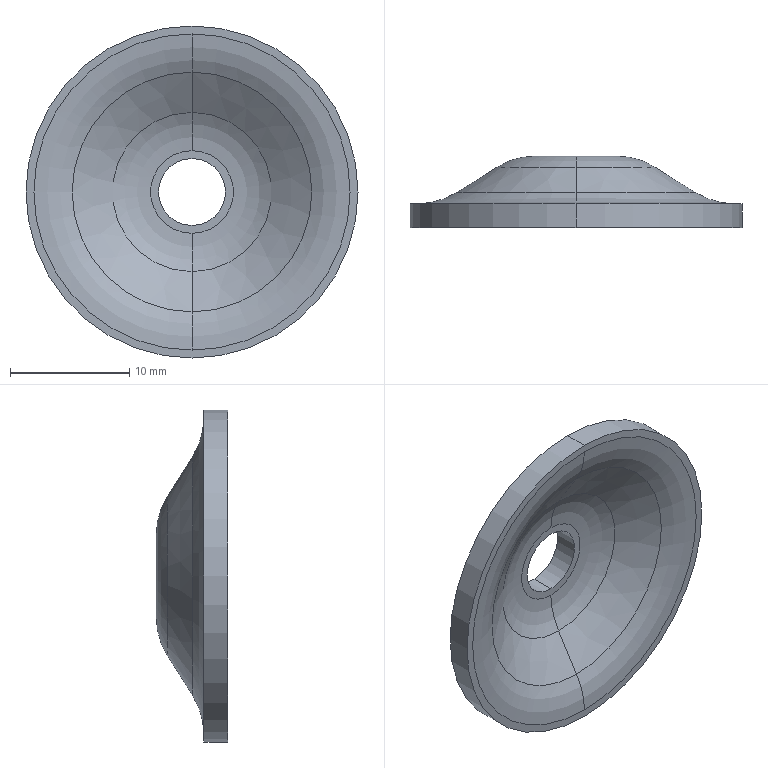Part | SolidWorks | features Revolution 1 | 1 solid | 20 faces | box 27.8 x 5.98 x 27.8 mm | volume 1165 mm3 | torus 8 | cone 4 | cylinder 4 | plane 4 | commonest cylinder face diameters 5.6 x2 27.8 x2
STEP:
#1=CARTESIAN_POINT('',(0.,-2.927,-6.668));
#2=VERTEX_POINT('',#1);
#3=CARTESIAN_POINT('',(0.,-2.927,6.668));
#4=VERTEX_POINT('',#3);
#5=CARTESIAN_POINT('',(0.,-2.927,0.));
#6=DIRECTION('',(0.,1.,0.));
#7=DIRECTION('',(0.,0.,1.));
#8=AXIS2_PLACEMENT_3D('',#5,#6,#7);
#9=CIRCLE('',#8,6.668);
#10=EDGE_CURVE('',#2,#4,#9,.T.);
#11=ORIENTED_EDGE('',*,*,#10,.F.);
#12=CARTESIAN_POINT('',(0.,-2.,-3.464));
#13=VERTEX_POINT('',#12);
#14=CARTESIAN_POINT('',(0.,-8.,-3.464));
#15=DIRECTION('',(1.,0.,0.));
#16=DIRECTION('',(0.,0.,-1.));
#17=AXIS2_PLACEMENT_3D('',#14,#15,#16);
#18=CIRCLE('',#17,6.);
#19=EDGE_CURVE('',#2,#13,#18,.T.);
#20=ORIENTED_EDGE('',*,*,#19,.T.);
#21=CARTESIAN_POINT('',(0.,-2.,3.464));
#22=VERTEX_POINT('',#21);
#23=CARTESIAN_POINT('',(0.,-2.,0.));
#24=DIRECTION('',(0.,1.,0.));
#25=DIRECTION('',(0.,0.,1.));
#26=AXIS2_PLACEMENT_3D('',#23,#24,#25);
#27=CIRCLE('',#26,3.464);
#28=EDGE_CURVE('',#13,#22,#27,.T.);
#29=ORIENTED_EDGE('',*,*,#28,.T.);
#30=CARTESIAN_POINT('',(0.,-8.,3.464));
#31=DIRECTION('',(-1.,0.,0.));
#32=DIRECTION('',(0.,0.,1.));
#33=AXIS2_PLACEMENT_3D('',#30,#31,#32);
#34=CIRCLE('',#33,6.);
#35=EDGE_CURVE('',#4,#22,#34,.T.);
#36=ORIENTED_EDGE('',*,*,#35,.F.);
#37=EDGE_LOOP('',(#11,#20,#29,#36));
#38=FACE_OUTER_BOUND('',#37,.T.);
#39=CARTESIAN_POINT('',(0.,-8.,0.));
#40=DIRECTION('',(0.,1.,0.));
#41=DIRECTION('',(0.,0.,1.));
#42=AXIS2_PLACEMENT_3D('',#39,#40,#41);
#43=TOROIDAL_SURFACE('',#42,3.464,6.);
#44=ADVANCED_FACE('',(#38),#43,.F.);
#45=ORIENTED_EDGE('',*,*,#10,.T.);
#46=CARTESIAN_POINT('',(0.,-5.053,10.032));
#47=VERTEX_POINT('',#46);
#48=CARTESIAN_POINT('',(0.,-5.053,10.032));
#49=DIRECTION('',(0.,-0.5341,0.8454));
#50=VECTOR('',#49,1000.);
#51=LINE('',#48,#50);
#52=EDGE_CURVE('',#4,#47,#51,.T.);
#53=ORIENTED_EDGE('',*,*,#52,.T.);
#54=CARTESIAN_POINT('',(0.,-5.053,-10.032));
#55=VERTEX_POINT('',#54);
#56=CARTESIAN_POINT('',(0.,-5.053,0.));
#57=DIRECTION('',(0.,1.,0.));
#58=DIRECTION('',(0.,0.,1.));
#59=AXIS2_PLACEMENT_3D('',#56,#57,#58);
#60=CIRCLE('',#59,10.032);
#61=EDGE_CURVE('',#55,#47,#60,.T.);
#62=ORIENTED_EDGE('',*,*,#61,.F.);
#63=CARTESIAN_POINT('',(0.,-5.053,-10.032));
#64=DIRECTION('',(0.,-0.5341,-0.8454));
#65=VECTOR('',#64,1000.);
#66=LINE('',#63,#65);
#67=EDGE_CURVE('',#2,#55,#66,.T.);
#68=ORIENTED_EDGE('',*,*,#67,.F.);
#69=EDGE_LOOP('',(#45,#53,#62,#68));
#70=FACE_OUTER_BOUND('',#69,.T.);
#71=CARTESIAN_POINT('',(0.,-5.053,0.));
#72=DIRECTION('',(0.,-1.,0.));
#73=DIRECTION('',(0.,0.,-1.));
#74=AXIS2_PLACEMENT_3D('',#71,#72,#73);
#75=CONICAL_SURFACE('',#74,10.032,1.007);
#76=ADVANCED_FACE('',(#70),#75,.F.);
#77=CARTESIAN_POINT('',(0.,-5.053,0.));
#78=DIRECTION('',(0.,1.,0.));
#79=DIRECTION('',(0.,0.,1.));
#80=AXIS2_PLACEMENT_3D('',#77,#78,#79);
#81=CIRCLE('',#80,10.032);
#82=EDGE_CURVE('',#47,#55,#81,.T.);
#83=ORIENTED_EDGE('',*,*,#82,.T.);
#84=CARTESIAN_POINT('',(0.,-5.98,-13.236));
#85=VERTEX_POINT('',#84);
#86=CARTESIAN_POINT('',(0.,0.02,-13.236));
#87=DIRECTION('',(1.,0.,0.));
#88=DIRECTION('',(0.,0.,-1.));
#89=AXIS2_PLACEMENT_3D('',#86,#87,#88);
#90=CIRCLE('',#89,6.);
#91=EDGE_CURVE('',#55,#85,#90,.T.);
#92=ORIENTED_EDGE('',*,*,#91,.T.);
#93=CARTESIAN_POINT('',(0.,-5.98,13.236));
#94=VERTEX_POINT('',#93);
#95=CARTESIAN_POINT('',(0.,-5.98,0.));
#96=DIRECTION('',(0.,1.,0.));
#97=DIRECTION('',(0.,0.,1.));
#98=AXIS2_PLACEMENT_3D('',#95,#96,#97);
#99=CIRCLE('',#98,13.236);
#100=EDGE_CURVE('',#94,#85,#99,.T.);
#101=ORIENTED_EDGE('',*,*,#100,.F.);
#102=CARTESIAN_POINT('',(0.,0.02,13.236));
#103=DIRECTION('',(-1.,0.,0.));
#104=DIRECTION('',(0.,0.,1.));
#105=AXIS2_PLACEMENT_3D('',#102,#103,#104);
#106=CIRCLE('',#105,6.);
#107=EDGE_CURVE('',#47,#94,#106,.T.);
#108=ORIENTED_EDGE('',*,*,#107,.F.);
#109=EDGE_LOOP('',(#83,#92,#101,#108));
#110=FACE_OUTER_BOUND('',#109,.T.);
#111=CARTESIAN_POINT('',(0.,0.02,0.));
#112=DIRECTION('',(0.,1.,0.));
#113=DIRECTION('',(0.,0.,1.));
#114=AXIS2_PLACEMENT_3D('',#111,#112,#113);
#115=TOROIDAL_SURFACE('',#114,13.236,6.);
#116=ADVANCED_FACE('',(#110),#115,.T.);
#117=CARTESIAN_POINT('',(0.,-5.98,13.9));
#118=VERTEX_POINT('',#117);
#119=CARTESIAN_POINT('',(0.,-5.98,-13.9));
#120=VERTEX_POINT('',#119);
#121=CARTESIAN_POINT('',(0.,-5.98,0.));
#122=DIRECTION('',(0.,1.,0.));
#123=DIRECTION('',(0.,0.,1.));
#124=AXIS2_PLACEMENT_3D('',#121,#122,#123);
#125=CIRCLE('',#124,13.9);
#126=EDGE_CURVE('',#118,#120,#125,.T.);
#127=ORIENTED_EDGE('',*,*,#126,.T.);
#128=CARTESIAN_POINT('',(0.,-3.98,-13.9));
#129=VERTEX_POINT('',#128);
#130=CARTESIAN_POINT('',(0.,0.,-13.9));
#131=DIRECTION('',(0.,1.,0.));
#132=VECTOR('',#131,1000.);
#133=LINE('',#130,#132);
#134=EDGE_CURVE('',#120,#129,#133,.T.);
#135=ORIENTED_EDGE('',*,*,#134,.T.);
#136=CARTESIAN_POINT('',(0.,-3.98,13.9));
#137=VERTEX_POINT('',#136);
#138=CARTESIAN_POINT('',(0.,-3.98,0.));
#139=DIRECTION('',(0.,1.,0.));
#140=DIRECTION('',(0.,0.,1.));
#141=AXIS2_PLACEMENT_3D('',#138,#139,#140);
#142=CIRCLE('',#141,13.9);
#143=EDGE_CURVE('',#137,#129,#142,.T.);
#144=ORIENTED_EDGE('',*,*,#143,.F.);
#145=CARTESIAN_POINT('',(0.,0.,13.9));
#146=DIRECTION('',(0.,1.,0.));
#147=VECTOR('',#146,1000.);
#148=LINE('',#145,#147);
#149=EDGE_CURVE('',#118,#137,#148,.T.);
#150=ORIENTED_EDGE('',*,*,#149,.F.);
#151=EDGE_LOOP('',(#127,#135,#144,#150));
#152=FACE_OUTER_BOUND('',#151,.T.);
#153=CARTESIAN_POINT('',(0.,0.,0.));
#154=DIRECTION('',(0.,1.,0.));
#155=DIRECTION('',(0.,0.,1.));
#156=AXIS2_PLACEMENT_3D('',#153,#154,#155);
#157=CYLINDRICAL_SURFACE('',#156,13.9);
#158=ADVANCED_FACE('',(#152),#157,.T.);
#159=CARTESIAN_POINT('',(0.,-3.053,-10.032));
#160=VERTEX_POINT('',#159);
#161=CARTESIAN_POINT('',(0.,-3.053,10.032));
#162=VERTEX_POINT('',#161);
#163=CARTESIAN_POINT('',(0.,-3.053,0.));
#164=DIRECTION('',(0.,1.,0.));
#165=DIRECTION('',(0.,0.,1.));
#166=AXIS2_PLACEMENT_3D('',#163,#164,#165);
#167=CIRCLE('',#166,10.032);
#168=EDGE_CURVE('',#160,#162,#167,.T.);
#169=ORIENTED_EDGE('',*,*,#168,.F.);
#170=CARTESIAN_POINT('',(0.,-3.98,-13.236));
#171=VERTEX_POINT('',#170);
#172=CARTESIAN_POINT('',(0.,2.02,-13.236));
#173=DIRECTION('',(1.,0.,0.));
#174=DIRECTION('',(0.,0.,-1.));
#175=AXIS2_PLACEMENT_3D('',#172,#173,#174);
#176=CIRCLE('',#175,6.);
#177=EDGE_CURVE('',#160,#171,#176,.T.);
#178=ORIENTED_EDGE('',*,*,#177,.T.);
#179=CARTESIAN_POINT('',(0.,-3.98,13.236));
#180=VERTEX_POINT('',#179);
#181=CARTESIAN_POINT('',(0.,-3.98,0.));
#182=DIRECTION('',(0.,1.,0.));
#183=DIRECTION('',(0.,0.,1.));
#184=AXIS2_PLACEMENT_3D('',#181,#182,#183);
#185=CIRCLE('',#184,13.236);
#186=EDGE_CURVE('',#171,#180,#185,.T.);
#187=ORIENTED_EDGE('',*,*,#186,.T.);
#188=CARTESIAN_POINT('',(0.,2.02,13.236));
#189=DIRECTION('',(-1.,0.,0.));
#190=DIRECTION('',(0.,0.,1.));
#191=AXIS2_PLACEMENT_3D('',#188,#189,#190);
#192=CIRCLE('',#191,6.);
#193=EDGE_CURVE('',#162,#180,#192,.T.);
#194=ORIENTED_EDGE('',*,*,#193,.F.);
#195=EDGE_LOOP('',(#169,#178,#187,#194));
#196=FACE_OUTER_BOUND('',#195,.T.);
#197=CARTESIAN_POINT('',(0.,2.02,0.));
#198=DIRECTION('',(0.,1.,0.));
#199=DIRECTION('',(0.,0.,1.));
#200=AXIS2_PLACEMENT_3D('',#197,#198,#199);
#201=TOROIDAL_SURFACE('',#200,13.236,6.);
#202=ADVANCED_FACE('',(#196),#201,.F.);
#203=CARTESIAN_POINT('',(0.,-0.9274,6.668));
#204=VERTEX_POINT('',#203);
#205=CARTESIAN_POINT('',(0.,-0.9274,-6.668));
#206=VERTEX_POINT('',#205);
#207=CARTESIAN_POINT('',(0.,-0.9274,0.));
#208=DIRECTION('',(0.,1.,0.));
#209=DIRECTION('',(0.,0.,1.));
#210=AXIS2_PLACEMENT_3D('',#207,#208,#209);
#211=CIRCLE('',#210,6.668);
#212=EDGE_CURVE('',#204,#206,#211,.T.);
#213=ORIENTED_EDGE('',*,*,#212,.F.);
#214=CARTESIAN_POINT('',(0.,-0.9274,6.668));
#215=DIRECTION('',(0.,-0.5341,0.8454));
#216=VECTOR('',#215,1000.);
#217=LINE('',#214,#216);
#218=EDGE_CURVE('',#204,#162,#217,.T.);
#219=ORIENTED_EDGE('',*,*,#218,.T.);
#220=CARTESIAN_POINT('',(0.,-3.053,0.));
#221=DIRECTION('',(0.,1.,0.));
#222=DIRECTION('',(0.,0.,1.));
#223=AXIS2_PLACEMENT_3D('',#220,#221,#222);
#224=CIRCLE('',#223,10.032);
#225=EDGE_CURVE('',#162,#160,#224,.T.);
#226=ORIENTED_EDGE('',*,*,#225,.T.);
#227=CARTESIAN_POINT('',(0.,-0.9274,-6.668));
#228=DIRECTION('',(0.,-0.5341,-0.8454));
#229=VECTOR('',#228,1000.);
#230=LINE('',#227,#229);
#231=EDGE_CURVE('',#206,#160,#230,.T.);
#232=ORIENTED_EDGE('',*,*,#231,.F.);
#233=EDGE_LOOP('',(#213,#219,#226,#232));
#234=FACE_OUTER_BOUND('',#233,.T.);
#235=CARTESIAN_POINT('',(0.,-0.9274,0.));
#236=DIRECTION('',(0.,-1.,0.));
#237=DIRECTION('',(0.,0.,-1.));
#238=AXIS2_PLACEMENT_3D('',#235,#236,#237);
#239=CONICAL_SURFACE('',#238,6.668,1.007);
#240=ADVANCED_FACE('',(#234),#239,.T.);
#241=ORIENTED_EDGE('',*,*,#212,.T.);
#242=CARTESIAN_POINT('',(0.,0.,-3.464));
#243=VERTEX_POINT('',#242);
#244=CARTESIAN_POINT('',(0.,-6.,-3.464));
#245=DIRECTION('',(1.,0.,0.));
#246=DIRECTION('',(0.,0.,-1.));
#247=AXIS2_PLACEMENT_3D('',#244,#245,#246);
#248=CIRCLE('',#247,6.);
#249=EDGE_CURVE('',#206,#243,#248,.T.);
#250=ORIENTED_EDGE('',*,*,#249,.T.);
#251=CARTESIAN_POINT('',(0.,0.,3.464));
#252=VERTEX_POINT('',#251);
#253=CARTESIAN_POINT('',(0.,0.,0.));
#254=DIRECTION('',(0.,1.,0.));
#255=DIRECTION('',(0.,0.,1.));
#256=AXIS2_PLACEMENT_3D('',#253,#254,#255);
#257=CIRCLE('',#256,3.464);
#258=EDGE_CURVE('',#252,#243,#257,.T.);
#259=ORIENTED_EDGE('',*,*,#258,.F.);
#260=CARTESIAN_POINT('',(0.,-6.,3.464));
#261=DIRECTION('',(-1.,0.,0.));
#262=DIRECTION('',(0.,0.,1.));
#263=AXIS2_PLACEMENT_3D('',#260,#261,#262);
#264=CIRCLE('',#263,6.);
#265=EDGE_CURVE('',#204,#252,#264,.T.);
#266=ORIENTED_EDGE('',*,*,#265,.F.);
#267=EDGE_LOOP('',(#241,#250,#259,#266));
#268=FACE_OUTER_BOUND('',#267,.T.);
#269=CARTESIAN_POINT('',(0.,-6.,0.));
#270=DIRECTION('',(0.,1.,0.));
#271=DIRECTION('',(0.,0.,1.));
#272=AXIS2_PLACEMENT_3D('',#269,#270,#271);
#273=TOROIDAL_SURFACE('',#272,3.464,6.);
#274=ADVANCED_FACE('',(#268),#273,.T.);
#275=CARTESIAN_POINT('',(0.,-2.,-2.8));
#276=VERTEX_POINT('',#275);
#277=CARTESIAN_POINT('',(0.,-2.,2.8));
#278=VERTEX_POINT('',#277);
#279=CARTESIAN_POINT('',(0.,-2.,0.));
#280=DIRECTION('',(0.,1.,0.));
#281=DIRECTION('',(0.,0.,1.));
#282=AXIS2_PLACEMENT_3D('',#279,#280,#281);
#283=CIRCLE('',#282,2.8);
#284=EDGE_CURVE('',#276,#278,#283,.T.);
#285=ORIENTED_EDGE('',*,*,#284,.F.);
#286=CARTESIAN_POINT('',(0.,0.,-2.8));
#287=VERTEX_POINT('',#286);
#288=CARTESIAN_POINT('',(0.,0.,-2.8));
#289=DIRECTION('',(0.,1.,0.));
#290=VECTOR('',#289,1000.);
#291=LINE('',#288,#290);
#292=EDGE_CURVE('',#276,#287,#291,.T.);
#293=ORIENTED_EDGE('',*,*,#292,.T.);
#294=CARTESIAN_POINT('',(0.,0.,2.8));
#295=VERTEX_POINT('',#294);
#296=CARTESIAN_POINT('',(0.,0.,0.));
#297=DIRECTION('',(0.,1.,0.));
#298=DIRECTION('',(0.,0.,1.));
#299=AXIS2_PLACEMENT_3D('',#296,#297,#298);
#300=CIRCLE('',#299,2.8);
#301=EDGE_CURVE('',#287,#295,#300,.T.);
#302=ORIENTED_EDGE('',*,*,#301,.T.);
#303=CARTESIAN_POINT('',(0.,0.,2.8));
#304=DIRECTION('',(0.,1.,0.));
#305=VECTOR('',#304,1000.);
#306=LINE('',#303,#305);
#307=EDGE_CURVE('',#278,#295,#306,.T.);
#308=ORIENTED_EDGE('',*,*,#307,.F.);
#309=EDGE_LOOP('',(#285,#293,#302,#308));
#310=FACE_OUTER_BOUND('',#309,.T.);
#311=CARTESIAN_POINT('',(0.,0.,0.));
#312=DIRECTION('',(0.,1.,0.));
#313=DIRECTION('',(0.,0.,1.));
#314=AXIS2_PLACEMENT_3D('',#311,#312,#313);
#315=CYLINDRICAL_SURFACE('',#314,2.8);
#316=ADVANCED_FACE('',(#310),#315,.F.);
#317=ORIENTED_EDGE('',*,*,#292,.F.);
#318=CARTESIAN_POINT('',(0.,-2.,0.));
#319=DIRECTION('',(0.,1.,0.));
#320=DIRECTION('',(0.,0.,1.));
#321=AXIS2_PLACEMENT_3D('',#318,#319,#320);
#322=CIRCLE('',#321,2.8);
#323=EDGE_CURVE('',#278,#276,#322,.T.);
#324=ORIENTED_EDGE('',*,*,#323,.F.);
#325=ORIENTED_EDGE('',*,*,#307,.T.);
#326=CARTESIAN_POINT('',(0.,0.,0.));
#327=DIRECTION('',(0.,1.,0.));
#328=DIRECTION('',(0.,0.,1.));
#329=AXIS2_PLACEMENT_3D('',#326,#327,#328);
#330=CIRCLE('',#329,2.8);
#331=EDGE_CURVE('',#295,#287,#330,.T.);
#332=ORIENTED_EDGE('',*,*,#331,.T.);
#333=EDGE_LOOP('',(#317,#324,#325,#332));
#334=FACE_OUTER_BOUND('',#333,.T.);
#335=CARTESIAN_POINT('',(0.,0.,0.));
#336=DIRECTION('',(0.,1.,0.));
#337=DIRECTION('',(0.,0.,1.));
#338=AXIS2_PLACEMENT_3D('',#335,#336,#337);
#339=CYLINDRICAL_SURFACE('',#338,2.8);
#340=ADVANCED_FACE('',(#334),#339,.F.);
#341=ORIENTED_EDGE('',*,*,#258,.T.);
#342=CARTESIAN_POINT('',(0.,0.,0.));
#343=DIRECTION('',(0.,1.,0.));
#344=DIRECTION('',(0.,0.,1.));
#345=AXIS2_PLACEMENT_3D('',#342,#343,#344);
#346=CIRCLE('',#345,3.464);
#347=EDGE_CURVE('',#243,#252,#346,.T.);
#348=ORIENTED_EDGE('',*,*,#347,.T.);
#349=EDGE_LOOP('',(#341,#348));
#350=FACE_OUTER_BOUND('',#349,.T.);
#351=ORIENTED_EDGE('',*,*,#331,.F.);
#352=ORIENTED_EDGE('',*,*,#301,.F.);
#353=EDGE_LOOP('',(#351,#352));
#354=FACE_BOUND('',#353,.T.);
#355=CARTESIAN_POINT('',(-2.8,0.,0.));
#356=DIRECTION('',(0.,1.,0.));
#357=DIRECTION('',(0.,0.,1.));
#358=AXIS2_PLACEMENT_3D('',#355,#356,#357);
#359=PLANE('',#358);
#360=ADVANCED_FACE('',(#350,#354),#359,.T.);
#361=ORIENTED_EDGE('',*,*,#249,.F.);
#362=CARTESIAN_POINT('',(0.,-0.9274,0.));
#363=DIRECTION('',(0.,1.,0.));
#364=DIRECTION('',(0.,0.,1.));
#365=AXIS2_PLACEMENT_3D('',#362,#363,#364);
#366=CIRCLE('',#365,6.668);
#367=EDGE_CURVE('',#206,#204,#366,.T.);
#368=ORIENTED_EDGE('',*,*,#367,.T.);
#369=ORIENTED_EDGE('',*,*,#265,.T.);
#370=ORIENTED_EDGE('',*,*,#347,.F.);
#371=EDGE_LOOP('',(#361,#368,#369,#370));
#372=FACE_OUTER_BOUND('',#371,.T.);
#373=CARTESIAN_POINT('',(0.,-6.,0.));
#374=DIRECTION('',(0.,1.,0.));
#375=DIRECTION('',(0.,0.,1.));
#376=AXIS2_PLACEMENT_3D('',#373,#374,#375);
#377=TOROIDAL_SURFACE('',#376,3.464,6.);
#378=ADVANCED_FACE('',(#372),#377,.T.);
#379=ORIENTED_EDGE('',*,*,#218,.F.);
#380=ORIENTED_EDGE('',*,*,#367,.F.);
#381=ORIENTED_EDGE('',*,*,#231,.T.);
#382=ORIENTED_EDGE('',*,*,#168,.T.);
#383=EDGE_LOOP('',(#379,#380,#381,#382));
#384=FACE_OUTER_BOUND('',#383,.T.);
#385=CARTESIAN_POINT('',(0.,-0.9274,0.));
#386=DIRECTION('',(0.,-1.,0.));
#387=DIRECTION('',(0.,0.,-1.));
#388=AXIS2_PLACEMENT_3D('',#385,#386,#387);
#389=CONICAL_SURFACE('',#388,6.668,1.007);
#390=ADVANCED_FACE('',(#384),#389,.T.);
#391=ORIENTED_EDGE('',*,*,#177,.F.);
#392=ORIENTED_EDGE('',*,*,#225,.F.);
#393=ORIENTED_EDGE('',*,*,#193,.T.);
#394=CARTESIAN_POINT('',(0.,-3.98,0.));
#395=DIRECTION('',(0.,1.,0.));
#396=DIRECTION('',(0.,0.,1.));
#397=AXIS2_PLACEMENT_3D('',#394,#395,#396);
#398=CIRCLE('',#397,13.236);
#399=EDGE_CURVE('',#180,#171,#398,.T.);
#400=ORIENTED_EDGE('',*,*,#399,.T.);
#401=EDGE_LOOP('',(#391,#392,#393,#400));
#402=FACE_OUTER_BOUND('',#401,.T.);
#403=CARTESIAN_POINT('',(0.,2.02,0.));
#404=DIRECTION('',(0.,1.,0.));
#405=DIRECTION('',(0.,0.,1.));
#406=AXIS2_PLACEMENT_3D('',#403,#404,#405);
#407=TOROIDAL_SURFACE('',#406,13.236,6.);
#408=ADVANCED_FACE('',(#402),#407,.F.);
#409=ORIENTED_EDGE('',*,*,#143,.T.);
#410=CARTESIAN_POINT('',(0.,-3.98,0.));
#411=DIRECTION('',(0.,1.,0.));
#412=DIRECTION('',(0.,0.,1.));
#413=AXIS2_PLACEMENT_3D('',#410,#411,#412);
#414=CIRCLE('',#413,13.9);
#415=EDGE_CURVE('',#129,#137,#414,.T.);
#416=ORIENTED_EDGE('',*,*,#415,.T.);
#417=EDGE_LOOP('',(#409,#416));
#418=FACE_OUTER_BOUND('',#417,.T.);
#419=ORIENTED_EDGE('',*,*,#399,.F.);
#420=ORIENTED_EDGE('',*,*,#186,.F.);
#421=EDGE_LOOP('',(#419,#420));
#422=FACE_BOUND('',#421,.T.);
#423=CARTESIAN_POINT('',(-13.236,-3.98,0.));
#424=DIRECTION('',(0.,1.,0.));
#425=DIRECTION('',(0.,0.,1.));
#426=AXIS2_PLACEMENT_3D('',#423,#424,#425);
#427=PLANE('',#426);
#428=ADVANCED_FACE('',(#418,#422),#427,.T.);
#429=ORIENTED_EDGE('',*,*,#134,.F.);
#430=CARTESIAN_POINT('',(0.,-5.98,0.));
#431=DIRECTION('',(0.,1.,0.));
#432=DIRECTION('',(0.,0.,1.));
#433=AXIS2_PLACEMENT_3D('',#430,#431,#432);
#434=CIRCLE('',#433,13.9);
#435=EDGE_CURVE('',#120,#118,#434,.T.);
#436=ORIENTED_EDGE('',*,*,#435,.T.);
#437=ORIENTED_EDGE('',*,*,#149,.T.);
#438=ORIENTED_EDGE('',*,*,#415,.F.);
#439=EDGE_LOOP('',(#429,#436,#437,#438));
#440=FACE_OUTER_BOUND('',#439,.T.);
#441=CARTESIAN_POINT('',(0.,0.,0.));
#442=DIRECTION('',(0.,1.,0.));
#443=DIRECTION('',(0.,0.,1.));
#444=AXIS2_PLACEMENT_3D('',#441,#442,#443);
#445=CYLINDRICAL_SURFACE('',#444,13.9);
#446=ADVANCED_FACE('',(#440),#445,.T.);
#447=ORIENTED_EDGE('',*,*,#100,.T.);
#448=CARTESIAN_POINT('',(0.,-5.98,0.));
#449=DIRECTION('',(0.,1.,0.));
#450=DIRECTION('',(0.,0.,1.));
#451=AXIS2_PLACEMENT_3D('',#448,#449,#450);
#452=CIRCLE('',#451,13.236);
#453=EDGE_CURVE('',#85,#94,#452,.T.);
#454=ORIENTED_EDGE('',*,*,#453,.T.);
#455=EDGE_LOOP('',(#447,#454));
#456=FACE_BOUND('',#455,.T.);
#457=ORIENTED_EDGE('',*,*,#126,.F.);
#458=ORIENTED_EDGE('',*,*,#435,.F.);
#459=EDGE_LOOP('',(#457,#458));
#460=FACE_OUTER_BOUND('',#459,.T.);
#461=CARTESIAN_POINT('',(-13.9,-5.98,0.));
#462=DIRECTION('',(0.,-1.,0.));
#463=DIRECTION('',(0.,0.,-1.));
#464=AXIS2_PLACEMENT_3D('',#461,#462,#463);
#465=PLANE('',#464);
#466=ADVANCED_FACE('',(#456,#460),#465,.T.);
#467=ORIENTED_EDGE('',*,*,#91,.F.);
#468=ORIENTED_EDGE('',*,*,#61,.T.);
#469=ORIENTED_EDGE('',*,*,#107,.T.);
#470=ORIENTED_EDGE('',*,*,#453,.F.);
#471=EDGE_LOOP('',(#467,#468,#469,#470));
#472=FACE_OUTER_BOUND('',#471,.T.);
#473=CARTESIAN_POINT('',(0.,0.02,0.));
#474=DIRECTION('',(0.,1.,0.));
#475=DIRECTION('',(0.,0.,1.));
#476=AXIS2_PLACEMENT_3D('',#473,#474,#475);
#477=TOROIDAL_SURFACE('',#476,13.236,6.);
#478=ADVANCED_FACE('',(#472),#477,.T.);
#479=ORIENTED_EDGE('',*,*,#52,.F.);
#480=CARTESIAN_POINT('',(0.,-2.927,0.));
#481=DIRECTION('',(0.,1.,0.));
#482=DIRECTION('',(0.,0.,1.));
#483=AXIS2_PLACEMENT_3D('',#480,#481,#482);
#484=CIRCLE('',#483,6.668);
#485=EDGE_CURVE('',#4,#2,#484,.T.);
#486=ORIENTED_EDGE('',*,*,#485,.T.);
#487=ORIENTED_EDGE('',*,*,#67,.T.);
#488=ORIENTED_EDGE('',*,*,#82,.F.);
#489=EDGE_LOOP('',(#479,#486,#487,#488));
#490=FACE_OUTER_BOUND('',#489,.T.);
#491=CARTESIAN_POINT('',(0.,-5.053,0.));
#492=DIRECTION('',(0.,-1.,0.));
#493=DIRECTION('',(0.,0.,-1.));
#494=AXIS2_PLACEMENT_3D('',#491,#492,#493);
#495=CONICAL_SURFACE('',#494,10.032,1.007);
#496=ADVANCED_FACE('',(#490),#495,.F.);
#497=ORIENTED_EDGE('',*,*,#19,.F.);
#498=ORIENTED_EDGE('',*,*,#485,.F.);
#499=ORIENTED_EDGE('',*,*,#35,.T.);
#500=CARTESIAN_POINT('',(0.,-2.,0.));
#501=DIRECTION('',(0.,1.,0.));
#502=DIRECTION('',(0.,0.,1.));
#503=AXIS2_PLACEMENT_3D('',#500,#501,#502);
#504=CIRCLE('',#503,3.464);
#505=EDGE_CURVE('',#22,#13,#504,.T.);
#506=ORIENTED_EDGE('',*,*,#505,.T.);
#507=EDGE_LOOP('',(#497,#498,#499,#506));
#508=FACE_OUTER_BOUND('',#507,.T.);
#509=CARTESIAN_POINT('',(0.,-8.,0.));
#510=DIRECTION('',(0.,1.,0.));
#511=DIRECTION('',(0.,0.,1.));
#512=AXIS2_PLACEMENT_3D('',#509,#510,#511);
#513=TOROIDAL_SURFACE('',#512,3.464,6.);
#514=ADVANCED_FACE('',(#508),#513,.F.);
#515=ORIENTED_EDGE('',*,*,#323,.T.);
#516=ORIENTED_EDGE('',*,*,#284,.T.);
#517=EDGE_LOOP('',(#515,#516));
#518=FACE_BOUND('',#517,.T.);
#519=ORIENTED_EDGE('',*,*,#505,.F.);
#520=ORIENTED_EDGE('',*,*,#28,.F.);
#521=EDGE_LOOP('',(#519,#520));
#522=FACE_OUTER_BOUND('',#521,.T.);
#523=CARTESIAN_POINT('',(-3.464,-2.,0.));
#524=DIRECTION('',(0.,-1.,0.));
#525=DIRECTION('',(0.,0.,-1.));
#526=AXIS2_PLACEMENT_3D('',#523,#524,#525);
#527=PLANE('',#526);
#528=ADVANCED_FACE('',(#518,#522),#527,.T.);
#529=CLOSED_SHELL('',(#44,#76,#116,#158,#202,#240,#274,#316,#340,#360,#378,#390,#408,#428,#446,#466,#478,#496,#514,#528));
#530=MANIFOLD_SOLID_BREP('',#529);
#531=CARTESIAN_POINT('',(0.,0.,0.));
#532=DIRECTION('',(0.,0.,1.));
#533=DIRECTION('',(1.,0.,0.));
#534=AXIS2_PLACEMENT_3D('',#531,#532,#533);
#535=(LENGTH_UNIT()NAMED_UNIT(*)SI_UNIT(.MILLI.,.METRE.));
#536=UNCERTAINTY_MEASURE_WITH_UNIT(LENGTH_MEASURE(0.00001),#535,'','');
#537=(NAMED_UNIT(*)PLANE_ANGLE_UNIT()SI_UNIT($,.RADIAN.));
#538=(NAMED_UNIT(*)SI_UNIT($,.STERADIAN.)SOLID_ANGLE_UNIT());
#539=(GEOMETRIC_REPRESENTATION_CONTEXT(3)GLOBAL_UNCERTAINTY_ASSIGNED_CONTEXT((#536))GLOBAL_UNIT_ASSIGNED_CONTEXT((#535,#537,#538))REPRESENTATION_CONTEXT('',''));
#540=ADVANCED_BREP_SHAPE_REPRESENTATION('',(#530,#534),#539);